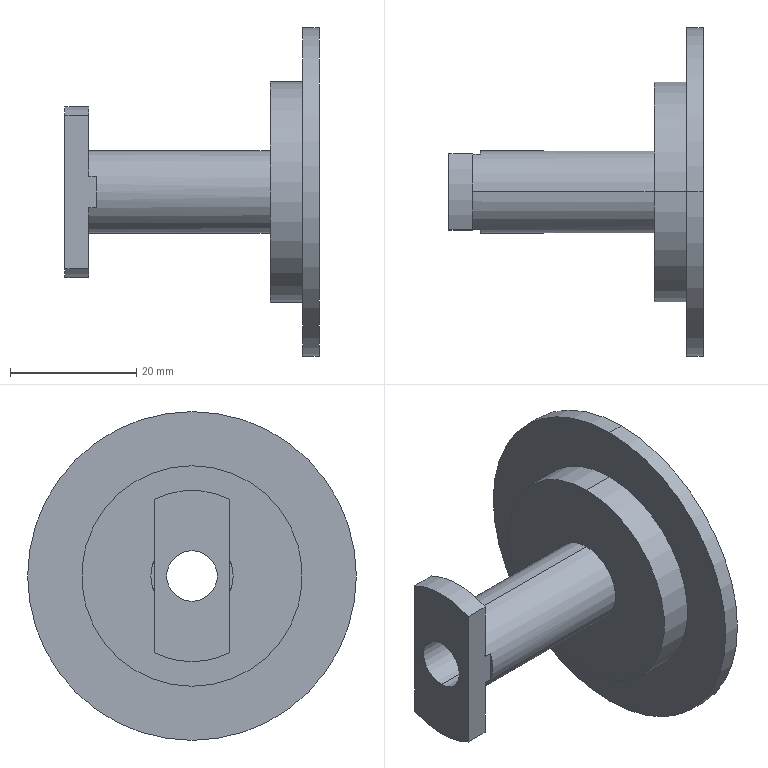Part | SolidWorks | features Cut 1, Revolution 1 | 1 solid | 24 faces | box 40.262 x 52.049 x 52.049 mm | volume 10319 mm3 | cylinder 13 | plane 11 | commonest cylinder face diameters 27.103 x3 8 x2 13.016 x2 28.307 x2 34.909 x2 52.049 x2
STEP:
#1=CARTESIAN_POINT('',(-77.,0.,14.154));
#2=VERTEX_POINT('',#1);
#3=CARTESIAN_POINT('',(-77.,0.,-14.154));
#4=VERTEX_POINT('',#3);
#5=CARTESIAN_POINT('',(-77.,0.,0.));
#6=DIRECTION('',(1.,0.,0.));
#7=DIRECTION('',(0.,0.,-1.));
#8=AXIS2_PLACEMENT_3D('',#5,#6,#7);
#9=CIRCLE('',#8,14.154);
#10=EDGE_CURVE('',#2,#4,#9,.T.);
#11=ORIENTED_EDGE('',*,*,#10,.F.);
#12=CARTESIAN_POINT('',(-71.527,0.,14.154));
#13=VERTEX_POINT('',#12);
#14=CARTESIAN_POINT('',(0.,0.,14.154));
#15=DIRECTION('',(1.,0.,0.));
#16=VECTOR('',#15,1000.);
#17=LINE('',#14,#16);
#18=EDGE_CURVE('',#2,#13,#17,.T.);
#19=ORIENTED_EDGE('',*,*,#18,.T.);
#20=CARTESIAN_POINT('',(-71.527,0.,-14.154));
#21=VERTEX_POINT('',#20);
#22=CARTESIAN_POINT('',(-71.527,0.,0.));
#23=DIRECTION('',(1.,0.,0.));
#24=DIRECTION('',(0.,0.,-1.));
#25=AXIS2_PLACEMENT_3D('',#22,#23,#24);
#26=CIRCLE('',#25,14.154);
#27=EDGE_CURVE('',#13,#21,#26,.T.);
#28=ORIENTED_EDGE('',*,*,#27,.T.);
#29=CARTESIAN_POINT('',(0.,0.,-14.154));
#30=DIRECTION('',(1.,0.,0.));
#31=VECTOR('',#30,1000.);
#32=LINE('',#29,#31);
#33=EDGE_CURVE('',#4,#21,#32,.T.);
#34=ORIENTED_EDGE('',*,*,#33,.F.);
#35=EDGE_LOOP('',(#11,#19,#28,#34));
#36=FACE_OUTER_BOUND('',#35,.T.);
#37=CARTESIAN_POINT('',(0.,0.,0.));
#38=DIRECTION('',(1.,0.,0.));
#39=DIRECTION('',(0.,0.,-1.));
#40=AXIS2_PLACEMENT_3D('',#37,#38,#39);
#41=CYLINDRICAL_SURFACE('',#40,14.154);
#42=ADVANCED_FACE('',(#36),#41,.F.);
#43=CARTESIAN_POINT('',(-111.789,0.,4.));
#44=VERTEX_POINT('',#43);
#45=CARTESIAN_POINT('',(-111.789,0.,-4.));
#46=VERTEX_POINT('',#45);
#47=CARTESIAN_POINT('',(-111.789,0.,0.));
#48=DIRECTION('',(1.,0.,0.));
#49=DIRECTION('',(0.,0.,-1.));
#50=AXIS2_PLACEMENT_3D('',#47,#48,#49);
#51=CIRCLE('',#50,4.);
#52=EDGE_CURVE('',#44,#46,#51,.T.);
#53=ORIENTED_EDGE('',*,*,#52,.F.);
#54=CARTESIAN_POINT('',(-77.,0.,4.));
#55=VERTEX_POINT('',#54);
#56=CARTESIAN_POINT('',(0.,0.,4.));
#57=DIRECTION('',(1.,0.,0.));
#58=VECTOR('',#57,1000.);
#59=LINE('',#56,#58);
#60=EDGE_CURVE('',#44,#55,#59,.T.);
#61=ORIENTED_EDGE('',*,*,#60,.T.);
#62=CARTESIAN_POINT('',(-77.,0.,-4.));
#63=VERTEX_POINT('',#62);
#64=CARTESIAN_POINT('',(-77.,0.,0.));
#65=DIRECTION('',(1.,0.,0.));
#66=DIRECTION('',(0.,0.,-1.));
#67=AXIS2_PLACEMENT_3D('',#64,#65,#66);
#68=CIRCLE('',#67,4.);
#69=EDGE_CURVE('',#55,#63,#68,.T.);
#70=ORIENTED_EDGE('',*,*,#69,.T.);
#71=CARTESIAN_POINT('',(0.,0.,-4.));
#72=DIRECTION('',(1.,0.,0.));
#73=VECTOR('',#72,1000.);
#74=LINE('',#71,#73);
#75=EDGE_CURVE('',#46,#63,#74,.T.);
#76=ORIENTED_EDGE('',*,*,#75,.F.);
#77=EDGE_LOOP('',(#53,#61,#70,#76));
#78=FACE_OUTER_BOUND('',#77,.T.);
#79=CARTESIAN_POINT('',(0.,0.,0.));
#80=DIRECTION('',(1.,0.,0.));
#81=DIRECTION('',(0.,0.,-1.));
#82=AXIS2_PLACEMENT_3D('',#79,#80,#81);
#83=CYLINDRICAL_SURFACE('',#82,4.);
#84=ADVANCED_FACE('',(#78),#83,.F.);
#85=CARTESIAN_POINT('',(-111.789,-6.,-12.151));
#86=VERTEX_POINT('',#85);
#87=CARTESIAN_POINT('',(-111.789,0.,-13.552));
#88=VERTEX_POINT('',#87);
#89=CARTESIAN_POINT('',(-111.789,0.,0.));
#90=DIRECTION('',(1.,0.,0.));
#91=DIRECTION('',(0.,0.,-1.));
#92=AXIS2_PLACEMENT_3D('',#89,#90,#91);
#93=CIRCLE('',#92,13.552);
#94=EDGE_CURVE('',#86,#88,#93,.T.);
#95=ORIENTED_EDGE('',*,*,#94,.T.);
#96=CARTESIAN_POINT('',(-108.,0.,-13.552));
#97=VERTEX_POINT('',#96);
#98=CARTESIAN_POINT('',(0.,0.,-13.552));
#99=DIRECTION('',(1.,0.,0.));
#100=VECTOR('',#99,1000.);
#101=LINE('',#98,#100);
#102=EDGE_CURVE('',#88,#97,#101,.T.);
#103=ORIENTED_EDGE('',*,*,#102,.T.);
#104=CARTESIAN_POINT('',(-108.,-6.,-12.151));
#105=VERTEX_POINT('',#104);
#106=CARTESIAN_POINT('',(-108.,0.,0.));
#107=DIRECTION('',(1.,0.,0.));
#108=DIRECTION('',(0.,0.,-1.));
#109=AXIS2_PLACEMENT_3D('',#106,#107,#108);
#110=CIRCLE('',#109,13.552);
#111=EDGE_CURVE('',#105,#97,#110,.T.);
#112=ORIENTED_EDGE('',*,*,#111,.F.);
#113=CARTESIAN_POINT('',(0.,-6.,-12.151));
#114=DIRECTION('',(1.,0.,0.));
#115=VECTOR('',#114,1000.);
#116=LINE('',#113,#115);
#117=EDGE_CURVE('',#86,#105,#116,.T.);
#118=ORIENTED_EDGE('',*,*,#117,.F.);
#119=EDGE_LOOP('',(#95,#103,#112,#118));
#120=FACE_OUTER_BOUND('',#119,.T.);
#121=CARTESIAN_POINT('',(0.,0.,0.));
#122=DIRECTION('',(1.,0.,0.));
#123=DIRECTION('',(0.,0.,-1.));
#124=AXIS2_PLACEMENT_3D('',#121,#122,#123);
#125=CYLINDRICAL_SURFACE('',#124,13.552);
#126=ADVANCED_FACE('',(#120),#125,.T.);
#127=CARTESIAN_POINT('',(-108.,6.,2.521));
#128=VERTEX_POINT('',#127);
#129=CARTESIAN_POINT('',(-108.,0.,6.508));
#130=VERTEX_POINT('',#129);
#131=CARTESIAN_POINT('',(-108.,0.,0.));
#132=DIRECTION('',(1.,0.,0.));
#133=DIRECTION('',(0.,0.,-1.));
#134=AXIS2_PLACEMENT_3D('',#131,#132,#133);
#135=CIRCLE('',#134,6.508);
#136=EDGE_CURVE('',#128,#130,#135,.T.);
#137=ORIENTED_EDGE('',*,*,#136,.T.);
#138=CARTESIAN_POINT('',(-79.307,0.,6.508));
#139=VERTEX_POINT('',#138);
#140=CARTESIAN_POINT('',(0.,0.,6.508));
#141=DIRECTION('',(1.,0.,0.));
#142=VECTOR('',#141,1000.);
#143=LINE('',#140,#142);
#144=EDGE_CURVE('',#130,#139,#143,.T.);
#145=ORIENTED_EDGE('',*,*,#144,.T.);
#146=CARTESIAN_POINT('',(-79.307,0.,-6.508));
#147=VERTEX_POINT('',#146);
#148=CARTESIAN_POINT('',(-79.307,0.,0.));
#149=DIRECTION('',(1.,0.,0.));
#150=DIRECTION('',(0.,0.,-1.));
#151=AXIS2_PLACEMENT_3D('',#148,#149,#150);
#152=CIRCLE('',#151,6.508);
#153=EDGE_CURVE('',#147,#139,#152,.T.);
#154=ORIENTED_EDGE('',*,*,#153,.F.);
#155=CARTESIAN_POINT('',(-108.,0.,-6.508));
#156=VERTEX_POINT('',#155);
#157=CARTESIAN_POINT('',(0.,0.,-6.508));
#158=DIRECTION('',(1.,0.,0.));
#159=VECTOR('',#158,1000.);
#160=LINE('',#157,#159);
#161=EDGE_CURVE('',#156,#147,#160,.T.);
#162=ORIENTED_EDGE('',*,*,#161,.F.);
#163=CARTESIAN_POINT('',(-108.,6.,-2.521));
#164=VERTEX_POINT('',#163);
#165=CARTESIAN_POINT('',(-108.,0.,0.));
#166=DIRECTION('',(1.,0.,0.));
#167=DIRECTION('',(0.,0.,-1.));
#168=AXIS2_PLACEMENT_3D('',#165,#166,#167);
#169=CIRCLE('',#168,6.508);
#170=EDGE_CURVE('',#156,#164,#169,.T.);
#171=ORIENTED_EDGE('',*,*,#170,.T.);
#172=CARTESIAN_POINT('',(-106.789,6.,-2.521));
#173=VERTEX_POINT('',#172);
#174=CARTESIAN_POINT('',(0.,6.,-2.521));
#175=DIRECTION('',(-1.,0.,0.));
#176=VECTOR('',#175,1000.);
#177=LINE('',#174,#176);
#178=EDGE_CURVE('',#173,#164,#177,.T.);
#179=ORIENTED_EDGE('',*,*,#178,.F.);
#180=CARTESIAN_POINT('',(-106.789,6.,2.521));
#181=VERTEX_POINT('',#180);
#182=CARTESIAN_POINT('',(-106.789,0.,0.));
#183=DIRECTION('',(1.,0.,0.));
#184=DIRECTION('',(0.,0.,1.));
#185=AXIS2_PLACEMENT_3D('',#182,#183,#184);
#186=CIRCLE('',#185,6.508);
#187=EDGE_CURVE('',#173,#181,#186,.T.);
#188=ORIENTED_EDGE('',*,*,#187,.T.);
#189=CARTESIAN_POINT('',(0.,6.,2.521));
#190=DIRECTION('',(1.,0.,0.));
#191=VECTOR('',#190,1000.);
#192=LINE('',#189,#191);
#193=EDGE_CURVE('',#128,#181,#192,.T.);
#194=ORIENTED_EDGE('',*,*,#193,.F.);
#195=EDGE_LOOP('',(#137,#145,#154,#162,#171,#179,#188,#194));
#196=FACE_OUTER_BOUND('',#195,.T.);
#197=CARTESIAN_POINT('',(0.,0.,0.));
#198=DIRECTION('',(1.,0.,0.));
#199=DIRECTION('',(0.,0.,-1.));
#200=AXIS2_PLACEMENT_3D('',#197,#198,#199);
#201=CYLINDRICAL_SURFACE('',#200,6.508);
#202=ADVANCED_FACE('',(#196),#201,.T.);
#203=CARTESIAN_POINT('',(-79.307,0.,-17.455));
#204=VERTEX_POINT('',#203);
#205=CARTESIAN_POINT('',(-79.307,0.,17.455));
#206=VERTEX_POINT('',#205);
#207=CARTESIAN_POINT('',(-79.307,0.,0.));
#208=DIRECTION('',(1.,0.,0.));
#209=DIRECTION('',(0.,0.,-1.));
#210=AXIS2_PLACEMENT_3D('',#207,#208,#209);
#211=CIRCLE('',#210,17.455);
#212=EDGE_CURVE('',#204,#206,#211,.T.);
#213=ORIENTED_EDGE('',*,*,#212,.T.);
#214=CARTESIAN_POINT('',(-74.143,0.,17.455));
#215=VERTEX_POINT('',#214);
#216=CARTESIAN_POINT('',(0.,0.,17.455));
#217=DIRECTION('',(1.,0.,0.));
#218=VECTOR('',#217,1000.);
#219=LINE('',#216,#218);
#220=EDGE_CURVE('',#206,#215,#219,.T.);
#221=ORIENTED_EDGE('',*,*,#220,.T.);
#222=CARTESIAN_POINT('',(-74.143,0.,-17.455));
#223=VERTEX_POINT('',#222);
#224=CARTESIAN_POINT('',(-74.143,0.,0.));
#225=DIRECTION('',(1.,0.,0.));
#226=DIRECTION('',(0.,0.,-1.));
#227=AXIS2_PLACEMENT_3D('',#224,#225,#226);
#228=CIRCLE('',#227,17.455);
#229=EDGE_CURVE('',#223,#215,#228,.T.);
#230=ORIENTED_EDGE('',*,*,#229,.F.);
#231=CARTESIAN_POINT('',(0.,0.,-17.455));
#232=DIRECTION('',(1.,0.,0.));
#233=VECTOR('',#232,1000.);
#234=LINE('',#231,#233);
#235=EDGE_CURVE('',#204,#223,#234,.T.);
#236=ORIENTED_EDGE('',*,*,#235,.F.);
#237=EDGE_LOOP('',(#213,#221,#230,#236));
#238=FACE_OUTER_BOUND('',#237,.T.);
#239=CARTESIAN_POINT('',(0.,0.,0.));
#240=DIRECTION('',(1.,0.,0.));
#241=DIRECTION('',(0.,0.,-1.));
#242=AXIS2_PLACEMENT_3D('',#239,#240,#241);
#243=CYLINDRICAL_SURFACE('',#242,17.455);
#244=ADVANCED_FACE('',(#238),#243,.T.);
#245=CARTESIAN_POINT('',(-74.143,0.,-26.024));
#246=VERTEX_POINT('',#245);
#247=CARTESIAN_POINT('',(-74.143,0.,26.024));
#248=VERTEX_POINT('',#247);
#249=CARTESIAN_POINT('',(-74.143,0.,0.));
#250=DIRECTION('',(1.,0.,0.));
#251=DIRECTION('',(0.,0.,-1.));
#252=AXIS2_PLACEMENT_3D('',#249,#250,#251);
#253=CIRCLE('',#252,26.024);
#254=EDGE_CURVE('',#246,#248,#253,.T.);
#255=ORIENTED_EDGE('',*,*,#254,.T.);
#256=CARTESIAN_POINT('',(-71.527,0.,26.024));
#257=VERTEX_POINT('',#256);
#258=CARTESIAN_POINT('',(0.,0.,26.024));
#259=DIRECTION('',(1.,0.,0.));
#260=VECTOR('',#259,1000.);
#261=LINE('',#258,#260);
#262=EDGE_CURVE('',#248,#257,#261,.T.);
#263=ORIENTED_EDGE('',*,*,#262,.T.);
#264=CARTESIAN_POINT('',(-71.527,0.,-26.024));
#265=VERTEX_POINT('',#264);
#266=CARTESIAN_POINT('',(-71.527,0.,0.));
#267=DIRECTION('',(1.,0.,0.));
#268=DIRECTION('',(0.,0.,-1.));
#269=AXIS2_PLACEMENT_3D('',#266,#267,#268);
#270=CIRCLE('',#269,26.024);
#271=EDGE_CURVE('',#265,#257,#270,.T.);
#272=ORIENTED_EDGE('',*,*,#271,.F.);
#273=CARTESIAN_POINT('',(0.,0.,-26.024));
#274=DIRECTION('',(1.,0.,0.));
#275=VECTOR('',#274,1000.);
#276=LINE('',#273,#275);
#277=EDGE_CURVE('',#246,#265,#276,.T.);
#278=ORIENTED_EDGE('',*,*,#277,.F.);
#279=EDGE_LOOP('',(#255,#263,#272,#278));
#280=FACE_OUTER_BOUND('',#279,.T.);
#281=CARTESIAN_POINT('',(0.,0.,0.));
#282=DIRECTION('',(1.,0.,0.));
#283=DIRECTION('',(0.,0.,-1.));
#284=AXIS2_PLACEMENT_3D('',#281,#282,#283);
#285=CYLINDRICAL_SURFACE('',#284,26.024);
#286=ADVANCED_FACE('',(#280),#285,.T.);
#287=CARTESIAN_POINT('',(-108.,-6.,-2.521));
#288=VERTEX_POINT('',#287);
#289=CARTESIAN_POINT('',(-108.,-6.,0.));
#290=DIRECTION('',(0.,0.,1.));
#291=VECTOR('',#290,1000.);
#292=LINE('',#289,#291);
#293=EDGE_CURVE('',#105,#288,#292,.T.);
#294=ORIENTED_EDGE('',*,*,#293,.F.);
#295=ORIENTED_EDGE('',*,*,#111,.T.);
#296=CARTESIAN_POINT('',(-108.,6.,-12.151));
#297=VERTEX_POINT('',#296);
#298=CARTESIAN_POINT('',(-108.,0.,0.));
#299=DIRECTION('',(1.,0.,0.));
#300=DIRECTION('',(0.,0.,-1.));
#301=AXIS2_PLACEMENT_3D('',#298,#299,#300);
#302=CIRCLE('',#301,13.552);
#303=EDGE_CURVE('',#97,#297,#302,.T.);
#304=ORIENTED_EDGE('',*,*,#303,.T.);
#305=CARTESIAN_POINT('',(-108.,6.,0.));
#306=DIRECTION('',(0.,0.,-1.));
#307=VECTOR('',#306,1000.);
#308=LINE('',#305,#307);
#309=EDGE_CURVE('',#164,#297,#308,.T.);
#310=ORIENTED_EDGE('',*,*,#309,.F.);
#311=ORIENTED_EDGE('',*,*,#170,.F.);
#312=CARTESIAN_POINT('',(-108.,0.,0.));
#313=DIRECTION('',(1.,0.,0.));
#314=DIRECTION('',(0.,0.,-1.));
#315=AXIS2_PLACEMENT_3D('',#312,#313,#314);
#316=CIRCLE('',#315,6.508);
#317=EDGE_CURVE('',#288,#156,#316,.T.);
#318=ORIENTED_EDGE('',*,*,#317,.F.);
#319=EDGE_LOOP('',(#294,#295,#304,#310,#311,#318));
#320=FACE_OUTER_BOUND('',#319,.T.);
#321=CARTESIAN_POINT('',(-108.,6.508,0.));
#322=DIRECTION('',(1.,0.,0.));
#323=DIRECTION('',(0.,0.,-1.));
#324=AXIS2_PLACEMENT_3D('',#321,#322,#323);
#325=PLANE('',#324);
#326=ADVANCED_FACE('',(#320),#325,.T.);
#327=CARTESIAN_POINT('',(-108.,-6.,12.151));
#328=VERTEX_POINT('',#327);
#329=CARTESIAN_POINT('',(-111.789,-6.,12.151));
#330=VERTEX_POINT('',#329);
#331=CARTESIAN_POINT('',(0.,-6.,12.151));
#332=DIRECTION('',(-1.,0.,0.));
#333=VECTOR('',#332,1000.);
#334=LINE('',#331,#333);
#335=EDGE_CURVE('',#328,#330,#334,.T.);
#336=ORIENTED_EDGE('',*,*,#335,.F.);
#337=CARTESIAN_POINT('',(-108.,6.,12.151));
#338=VERTEX_POINT('',#337);
#339=CARTESIAN_POINT('',(-108.,0.,0.));
#340=DIRECTION('',(1.,0.,0.));
#341=DIRECTION('',(0.,0.,-1.));
#342=AXIS2_PLACEMENT_3D('',#339,#340,#341);
#343=CIRCLE('',#342,13.552);
#344=EDGE_CURVE('',#338,#328,#343,.T.);
#345=ORIENTED_EDGE('',*,*,#344,.F.);
#346=CARTESIAN_POINT('',(-111.789,6.,12.151));
#347=VERTEX_POINT('',#346);
#348=CARTESIAN_POINT('',(0.,6.,12.151));
#349=DIRECTION('',(1.,0.,0.));
#350=VECTOR('',#349,1000.);
#351=LINE('',#348,#350);
#352=EDGE_CURVE('',#347,#338,#351,.T.);
#353=ORIENTED_EDGE('',*,*,#352,.F.);
#354=CARTESIAN_POINT('',(-111.789,0.,0.));
#355=DIRECTION('',(1.,0.,0.));
#356=DIRECTION('',(0.,0.,-1.));
#357=AXIS2_PLACEMENT_3D('',#354,#355,#356);
#358=CIRCLE('',#357,13.552);
#359=EDGE_CURVE('',#347,#330,#358,.T.);
#360=ORIENTED_EDGE('',*,*,#359,.T.);
#361=EDGE_LOOP('',(#336,#345,#353,#360));
#362=FACE_OUTER_BOUND('',#361,.T.);
#363=CARTESIAN_POINT('',(0.,0.,0.));
#364=DIRECTION('',(1.,0.,0.));
#365=DIRECTION('',(0.,0.,-1.));
#366=AXIS2_PLACEMENT_3D('',#363,#364,#365);
#367=CYLINDRICAL_SURFACE('',#366,13.552);
#368=ADVANCED_FACE('',(#362),#367,.T.);
#369=ORIENTED_EDGE('',*,*,#262,.F.);
#370=CARTESIAN_POINT('',(-74.143,0.,0.));
#371=DIRECTION('',(1.,0.,0.));
#372=DIRECTION('',(0.,0.,-1.));
#373=AXIS2_PLACEMENT_3D('',#370,#371,#372);
#374=CIRCLE('',#373,26.024);
#375=EDGE_CURVE('',#248,#246,#374,.T.);
#376=ORIENTED_EDGE('',*,*,#375,.T.);
#377=ORIENTED_EDGE('',*,*,#277,.T.);
#378=CARTESIAN_POINT('',(-71.527,0.,0.));
#379=DIRECTION('',(1.,0.,0.));
#380=DIRECTION('',(0.,0.,-1.));
#381=AXIS2_PLACEMENT_3D('',#378,#379,#380);
#382=CIRCLE('',#381,26.024);
#383=EDGE_CURVE('',#257,#265,#382,.T.);
#384=ORIENTED_EDGE('',*,*,#383,.F.);
#385=EDGE_LOOP('',(#369,#376,#377,#384));
#386=FACE_OUTER_BOUND('',#385,.T.);
#387=CARTESIAN_POINT('',(0.,0.,0.));
#388=DIRECTION('',(1.,0.,0.));
#389=DIRECTION('',(0.,0.,-1.));
#390=AXIS2_PLACEMENT_3D('',#387,#388,#389);
#391=CYLINDRICAL_SURFACE('',#390,26.024);
#392=ADVANCED_FACE('',(#386),#391,.T.);
#393=ORIENTED_EDGE('',*,*,#229,.T.);
#394=CARTESIAN_POINT('',(-74.143,0.,0.));
#395=DIRECTION('',(1.,0.,0.));
#396=DIRECTION('',(0.,0.,-1.));
#397=AXIS2_PLACEMENT_3D('',#394,#395,#396);
#398=CIRCLE('',#397,17.455);
#399=EDGE_CURVE('',#215,#223,#398,.T.);
#400=ORIENTED_EDGE('',*,*,#399,.T.);
#401=EDGE_LOOP('',(#393,#400));
#402=FACE_BOUND('',#401,.T.);
#403=ORIENTED_EDGE('',*,*,#254,.F.);
#404=ORIENTED_EDGE('',*,*,#375,.F.);
#405=EDGE_LOOP('',(#403,#404));
#406=FACE_OUTER_BOUND('',#405,.T.);
#407=CARTESIAN_POINT('',(-74.143,26.024,0.));
#408=DIRECTION('',(-1.,0.,0.));
#409=DIRECTION('',(0.,0.,1.));
#410=AXIS2_PLACEMENT_3D('',#407,#408,#409);
#411=PLANE('',#410);
#412=ADVANCED_FACE('',(#402,#406),#411,.T.);
#413=ORIENTED_EDGE('',*,*,#220,.F.);
#414=CARTESIAN_POINT('',(-79.307,0.,0.));
#415=DIRECTION('',(1.,0.,0.));
#416=DIRECTION('',(0.,0.,-1.));
#417=AXIS2_PLACEMENT_3D('',#414,#415,#416);
#418=CIRCLE('',#417,17.455);
#419=EDGE_CURVE('',#206,#204,#418,.T.);
#420=ORIENTED_EDGE('',*,*,#419,.T.);
#421=ORIENTED_EDGE('',*,*,#235,.T.);
#422=ORIENTED_EDGE('',*,*,#399,.F.);
#423=EDGE_LOOP('',(#413,#420,#421,#422));
#424=FACE_OUTER_BOUND('',#423,.T.);
#425=CARTESIAN_POINT('',(0.,0.,0.));
#426=DIRECTION('',(1.,0.,0.));
#427=DIRECTION('',(0.,0.,-1.));
#428=AXIS2_PLACEMENT_3D('',#425,#426,#427);
#429=CYLINDRICAL_SURFACE('',#428,17.455);
#430=ADVANCED_FACE('',(#424),#429,.T.);
#431=ORIENTED_EDGE('',*,*,#153,.T.);
#432=CARTESIAN_POINT('',(-79.307,0.,0.));
#433=DIRECTION('',(1.,0.,0.));
#434=DIRECTION('',(0.,0.,-1.));
#435=AXIS2_PLACEMENT_3D('',#432,#433,#434);
#436=CIRCLE('',#435,6.508);
#437=EDGE_CURVE('',#139,#147,#436,.T.);
#438=ORIENTED_EDGE('',*,*,#437,.T.);
#439=EDGE_LOOP('',(#431,#438));
#440=FACE_BOUND('',#439,.T.);
#441=ORIENTED_EDGE('',*,*,#212,.F.);
#442=ORIENTED_EDGE('',*,*,#419,.F.);
#443=EDGE_LOOP('',(#441,#442));
#444=FACE_OUTER_BOUND('',#443,.T.);
#445=CARTESIAN_POINT('',(-79.307,17.455,0.));
#446=DIRECTION('',(-1.,0.,0.));
#447=DIRECTION('',(0.,0.,1.));
#448=AXIS2_PLACEMENT_3D('',#445,#446,#447);
#449=PLANE('',#448);
#450=ADVANCED_FACE('',(#440,#444),#449,.T.);
#451=ORIENTED_EDGE('',*,*,#144,.F.);
#452=CARTESIAN_POINT('',(-108.,-6.,2.521));
#453=VERTEX_POINT('',#452);
#454=CARTESIAN_POINT('',(-108.,0.,0.));
#455=DIRECTION('',(1.,0.,0.));
#456=DIRECTION('',(0.,0.,-1.));
#457=AXIS2_PLACEMENT_3D('',#454,#455,#456);
#458=CIRCLE('',#457,6.508);
#459=EDGE_CURVE('',#130,#453,#458,.T.);
#460=ORIENTED_EDGE('',*,*,#459,.T.);
#461=CARTESIAN_POINT('',(-106.789,-6.,2.521));
#462=VERTEX_POINT('',#461);
#463=CARTESIAN_POINT('',(0.,-6.,2.521));
#464=DIRECTION('',(-1.,0.,0.));
#465=VECTOR('',#464,1000.);
#466=LINE('',#463,#465);
#467=EDGE_CURVE('',#462,#453,#466,.T.);
#468=ORIENTED_EDGE('',*,*,#467,.F.);
#469=CARTESIAN_POINT('',(-106.789,-6.,-2.521));
#470=VERTEX_POINT('',#469);
#471=CARTESIAN_POINT('',(-106.789,0.,0.));
#472=DIRECTION('',(-1.,0.,0.));
#473=DIRECTION('',(0.,0.,-1.));
#474=AXIS2_PLACEMENT_3D('',#471,#472,#473);
#475=CIRCLE('',#474,6.508);
#476=EDGE_CURVE('',#470,#462,#475,.T.);
#477=ORIENTED_EDGE('',*,*,#476,.F.);
#478=CARTESIAN_POINT('',(0.,-6.,-2.521));
#479=DIRECTION('',(1.,0.,0.));
#480=VECTOR('',#479,1000.);
#481=LINE('',#478,#480);
#482=EDGE_CURVE('',#288,#470,#481,.T.);
#483=ORIENTED_EDGE('',*,*,#482,.F.);
#484=ORIENTED_EDGE('',*,*,#317,.T.);
#485=ORIENTED_EDGE('',*,*,#161,.T.);
#486=ORIENTED_EDGE('',*,*,#437,.F.);
#487=EDGE_LOOP('',(#451,#460,#468,#477,#483,#484,#485,#486));
#488=FACE_OUTER_BOUND('',#487,.T.);
#489=CARTESIAN_POINT('',(0.,0.,0.));
#490=DIRECTION('',(1.,0.,0.));
#491=DIRECTION('',(0.,0.,-1.));
#492=AXIS2_PLACEMENT_3D('',#489,#490,#491);
#493=CYLINDRICAL_SURFACE('',#492,6.508);
#494=ADVANCED_FACE('',(#488),#493,.T.);
#495=CARTESIAN_POINT('',(-108.,-6.,0.));
#496=DIRECTION('',(0.,0.,1.));
#497=VECTOR('',#496,1000.);
#498=LINE('',#495,#497);
#499=EDGE_CURVE('',#453,#328,#498,.T.);
#500=ORIENTED_EDGE('',*,*,#499,.F.);
#501=ORIENTED_EDGE('',*,*,#459,.F.);
#502=ORIENTED_EDGE('',*,*,#136,.F.);
#503=CARTESIAN_POINT('',(-108.,6.,0.));
#504=DIRECTION('',(0.,0.,-1.));
#505=VECTOR('',#504,1000.);
#506=LINE('',#503,#505);
#507=EDGE_CURVE('',#338,#128,#506,.T.);
#508=ORIENTED_EDGE('',*,*,#507,.F.);
#509=ORIENTED_EDGE('',*,*,#344,.T.);
#510=EDGE_LOOP('',(#500,#501,#502,#508,#509));
#511=FACE_OUTER_BOUND('',#510,.T.);
#512=CARTESIAN_POINT('',(-108.,6.508,0.));
#513=DIRECTION('',(1.,0.,0.));
#514=DIRECTION('',(0.,0.,-1.));
#515=AXIS2_PLACEMENT_3D('',#512,#513,#514);
#516=PLANE('',#515);
#517=ADVANCED_FACE('',(#511),#516,.T.);
#518=ORIENTED_EDGE('',*,*,#102,.F.);
#519=CARTESIAN_POINT('',(-111.789,6.,-12.151));
#520=VERTEX_POINT('',#519);
#521=CARTESIAN_POINT('',(-111.789,0.,0.));
#522=DIRECTION('',(1.,0.,0.));
#523=DIRECTION('',(0.,0.,-1.));
#524=AXIS2_PLACEMENT_3D('',#521,#522,#523);
#525=CIRCLE('',#524,13.552);
#526=EDGE_CURVE('',#88,#520,#525,.T.);
#527=ORIENTED_EDGE('',*,*,#526,.T.);
#528=CARTESIAN_POINT('',(0.,6.,-12.151));
#529=DIRECTION('',(-1.,0.,0.));
#530=VECTOR('',#529,1000.);
#531=LINE('',#528,#530);
#532=EDGE_CURVE('',#297,#520,#531,.T.);
#533=ORIENTED_EDGE('',*,*,#532,.F.);
#534=ORIENTED_EDGE('',*,*,#303,.F.);
#535=EDGE_LOOP('',(#518,#527,#533,#534));
#536=FACE_OUTER_BOUND('',#535,.T.);
#537=CARTESIAN_POINT('',(0.,0.,0.));
#538=DIRECTION('',(1.,0.,0.));
#539=DIRECTION('',(0.,0.,-1.));
#540=AXIS2_PLACEMENT_3D('',#537,#538,#539);
#541=CYLINDRICAL_SURFACE('',#540,13.552);
#542=ADVANCED_FACE('',(#536),#541,.T.);
#543=CARTESIAN_POINT('',(-111.789,-6.,0.));
#544=DIRECTION('',(0.,0.,-1.));
#545=VECTOR('',#544,1000.);
#546=LINE('',#543,#545);
#547=EDGE_CURVE('',#330,#86,#546,.T.);
#548=ORIENTED_EDGE('',*,*,#547,.F.);
#549=ORIENTED_EDGE('',*,*,#359,.F.);
#550=CARTESIAN_POINT('',(-111.789,6.,0.));
#551=DIRECTION('',(0.,0.,1.));
#552=VECTOR('',#551,1000.);
#553=LINE('',#550,#552);
#554=EDGE_CURVE('',#520,#347,#553,.T.);
#555=ORIENTED_EDGE('',*,*,#554,.F.);
#556=ORIENTED_EDGE('',*,*,#526,.F.);
#557=ORIENTED_EDGE('',*,*,#94,.F.);
#558=EDGE_LOOP('',(#548,#549,#555,#556,#557));
#559=FACE_OUTER_BOUND('',#558,.T.);
#560=CARTESIAN_POINT('',(-111.789,0.,0.));
#561=DIRECTION('',(1.,0.,0.));
#562=DIRECTION('',(0.,0.,-1.));
#563=AXIS2_PLACEMENT_3D('',#560,#561,#562);
#564=CIRCLE('',#563,4.);
#565=EDGE_CURVE('',#46,#44,#564,.T.);
#566=ORIENTED_EDGE('',*,*,#565,.T.);
#567=ORIENTED_EDGE('',*,*,#52,.T.);
#568=EDGE_LOOP('',(#566,#567));
#569=FACE_BOUND('',#568,.T.);
#570=CARTESIAN_POINT('',(-111.789,13.552,0.));
#571=DIRECTION('',(-1.,0.,0.));
#572=DIRECTION('',(0.,0.,1.));
#573=AXIS2_PLACEMENT_3D('',#570,#571,#572);
#574=PLANE('',#573);
#575=ADVANCED_FACE('',(#559,#569),#574,.T.);
#576=ORIENTED_EDGE('',*,*,#60,.F.);
#577=ORIENTED_EDGE('',*,*,#565,.F.);
#578=ORIENTED_EDGE('',*,*,#75,.T.);
#579=CARTESIAN_POINT('',(-77.,0.,0.));
#580=DIRECTION('',(1.,0.,0.));
#581=DIRECTION('',(0.,0.,-1.));
#582=AXIS2_PLACEMENT_3D('',#579,#580,#581);
#583=CIRCLE('',#582,4.);
#584=EDGE_CURVE('',#63,#55,#583,.T.);
#585=ORIENTED_EDGE('',*,*,#584,.T.);
#586=EDGE_LOOP('',(#576,#577,#578,#585));
#587=FACE_OUTER_BOUND('',#586,.T.);
#588=CARTESIAN_POINT('',(0.,0.,0.));
#589=DIRECTION('',(1.,0.,0.));
#590=DIRECTION('',(0.,0.,-1.));
#591=AXIS2_PLACEMENT_3D('',#588,#589,#590);
#592=CYLINDRICAL_SURFACE('',#591,4.);
#593=ADVANCED_FACE('',(#587),#592,.F.);
#594=CARTESIAN_POINT('',(-77.,0.,0.));
#595=DIRECTION('',(1.,0.,0.));
#596=DIRECTION('',(0.,0.,-1.));
#597=AXIS2_PLACEMENT_3D('',#594,#595,#596);
#598=CIRCLE('',#597,14.154);
#599=EDGE_CURVE('',#4,#2,#598,.T.);
#600=ORIENTED_EDGE('',*,*,#599,.T.);
#601=ORIENTED_EDGE('',*,*,#10,.T.);
#602=EDGE_LOOP('',(#600,#601));
#603=FACE_OUTER_BOUND('',#602,.T.);
#604=ORIENTED_EDGE('',*,*,#584,.F.);
#605=ORIENTED_EDGE('',*,*,#69,.F.);
#606=EDGE_LOOP('',(#604,#605));
#607=FACE_BOUND('',#606,.T.);
#608=CARTESIAN_POINT('',(-77.,4.,0.));
#609=DIRECTION('',(1.,0.,0.));
#610=DIRECTION('',(0.,0.,-1.));
#611=AXIS2_PLACEMENT_3D('',#608,#609,#610);
#612=PLANE('',#611);
#613=ADVANCED_FACE('',(#603,#607),#612,.T.);
#614=ORIENTED_EDGE('',*,*,#18,.F.);
#615=ORIENTED_EDGE('',*,*,#599,.F.);
#616=ORIENTED_EDGE('',*,*,#33,.T.);
#617=CARTESIAN_POINT('',(-71.527,0.,0.));
#618=DIRECTION('',(1.,0.,0.));
#619=DIRECTION('',(0.,0.,-1.));
#620=AXIS2_PLACEMENT_3D('',#617,#618,#619);
#621=CIRCLE('',#620,14.154);
#622=EDGE_CURVE('',#21,#13,#621,.T.);
#623=ORIENTED_EDGE('',*,*,#622,.T.);
#624=EDGE_LOOP('',(#614,#615,#616,#623));
#625=FACE_OUTER_BOUND('',#624,.T.);
#626=CARTESIAN_POINT('',(0.,0.,0.));
#627=DIRECTION('',(1.,0.,0.));
#628=DIRECTION('',(0.,0.,-1.));
#629=AXIS2_PLACEMENT_3D('',#626,#627,#628);
#630=CYLINDRICAL_SURFACE('',#629,14.154);
#631=ADVANCED_FACE('',(#625),#630,.F.);
#632=ORIENTED_EDGE('',*,*,#271,.T.);
#633=ORIENTED_EDGE('',*,*,#383,.T.);
#634=EDGE_LOOP('',(#632,#633));
#635=FACE_OUTER_BOUND('',#634,.T.);
#636=ORIENTED_EDGE('',*,*,#622,.F.);
#637=ORIENTED_EDGE('',*,*,#27,.F.);
#638=EDGE_LOOP('',(#636,#637));
#639=FACE_BOUND('',#638,.T.);
#640=CARTESIAN_POINT('',(-71.527,14.154,0.));
#641=DIRECTION('',(1.,0.,0.));
#642=DIRECTION('',(0.,0.,-1.));
#643=AXIS2_PLACEMENT_3D('',#640,#641,#642);
#644=PLANE('',#643);
#645=ADVANCED_FACE('',(#635,#639),#644,.T.);
#646=ORIENTED_EDGE('',*,*,#178,.T.);
#647=ORIENTED_EDGE('',*,*,#309,.T.);
#648=ORIENTED_EDGE('',*,*,#532,.T.);
#649=ORIENTED_EDGE('',*,*,#554,.T.);
#650=ORIENTED_EDGE('',*,*,#352,.T.);
#651=ORIENTED_EDGE('',*,*,#507,.T.);
#652=ORIENTED_EDGE('',*,*,#193,.T.);
#653=CARTESIAN_POINT('',(-106.789,6.,-44.604));
#654=DIRECTION('',(0.,0.,1.));
#655=VECTOR('',#654,1000.);
#656=LINE('',#653,#655);
#657=EDGE_CURVE('',#173,#181,#656,.T.);
#658=ORIENTED_EDGE('',*,*,#657,.F.);
#659=EDGE_LOOP('',(#646,#647,#648,#649,#650,#651,#652,#658));
#660=FACE_OUTER_BOUND('',#659,.T.);
#661=CARTESIAN_POINT('',(-106.789,6.,-44.604));
#662=DIRECTION('',(0.,-1.,0.));
#663=DIRECTION('',(0.,0.,-1.));
#664=AXIS2_PLACEMENT_3D('',#661,#662,#663);
#665=PLANE('',#664);
#666=ADVANCED_FACE('',(#660),#665,.F.);
#667=ORIENTED_EDGE('',*,*,#657,.T.);
#668=ORIENTED_EDGE('',*,*,#187,.F.);
#669=EDGE_LOOP('',(#667,#668));
#670=FACE_OUTER_BOUND('',#669,.T.);
#671=CARTESIAN_POINT('',(-106.789,0.,0.));
#672=DIRECTION('',(-1.,0.,0.));
#673=DIRECTION('',(0.,0.,1.));
#674=AXIS2_PLACEMENT_3D('',#671,#672,#673);
#675=PLANE('',#674);
#676=ADVANCED_FACE('',(#670),#675,.T.);
#677=ORIENTED_EDGE('',*,*,#467,.T.);
#678=ORIENTED_EDGE('',*,*,#499,.T.);
#679=ORIENTED_EDGE('',*,*,#335,.T.);
#680=ORIENTED_EDGE('',*,*,#547,.T.);
#681=ORIENTED_EDGE('',*,*,#117,.T.);
#682=ORIENTED_EDGE('',*,*,#293,.T.);
#683=ORIENTED_EDGE('',*,*,#482,.T.);
#684=CARTESIAN_POINT('',(-106.789,-6.,79.996));
#685=DIRECTION('',(0.,0.,-1.));
#686=VECTOR('',#685,1000.);
#687=LINE('',#684,#686);
#688=EDGE_CURVE('',#462,#470,#687,.T.);
#689=ORIENTED_EDGE('',*,*,#688,.F.);
#690=EDGE_LOOP('',(#677,#678,#679,#680,#681,#682,#683,#689));
#691=FACE_OUTER_BOUND('',#690,.T.);
#692=CARTESIAN_POINT('',(-106.789,-6.,79.996));
#693=DIRECTION('',(0.,1.,0.));
#694=DIRECTION('',(0.,0.,1.));
#695=AXIS2_PLACEMENT_3D('',#692,#693,#694);
#696=PLANE('',#695);
#697=ADVANCED_FACE('',(#691),#696,.F.);
#698=ORIENTED_EDGE('',*,*,#476,.T.);
#699=ORIENTED_EDGE('',*,*,#688,.T.);
#700=EDGE_LOOP('',(#698,#699));
#701=FACE_OUTER_BOUND('',#700,.T.);
#702=CARTESIAN_POINT('',(-106.789,0.,0.));
#703=DIRECTION('',(1.,0.,0.));
#704=DIRECTION('',(0.,0.,-1.));
#705=AXIS2_PLACEMENT_3D('',#702,#703,#704);
#706=PLANE('',#705);
#707=ADVANCED_FACE('',(#701),#706,.F.);
#708=CLOSED_SHELL('',(#42,#84,#126,#202,#244,#286,#326,#368,#392,#412,#430,#450,#494,#517,#542,#575,#593,#613,#631,#645,#666,#676,#697,#707));
#709=MANIFOLD_SOLID_BREP('',#708);
#710=CARTESIAN_POINT('',(0.,0.,0.));
#711=DIRECTION('',(0.,0.,1.));
#712=DIRECTION('',(1.,0.,0.));
#713=AXIS2_PLACEMENT_3D('',#710,#711,#712);
#714=(LENGTH_UNIT()NAMED_UNIT(*)SI_UNIT(.MILLI.,.METRE.));
#715=UNCERTAINTY_MEASURE_WITH_UNIT(LENGTH_MEASURE(0.00001),#714,'','');
#716=(NAMED_UNIT(*)PLANE_ANGLE_UNIT()SI_UNIT($,.RADIAN.));
#717=(NAMED_UNIT(*)SI_UNIT($,.STERADIAN.)SOLID_ANGLE_UNIT());
#718=(GEOMETRIC_REPRESENTATION_CONTEXT(3)GLOBAL_UNCERTAINTY_ASSIGNED_CONTEXT((#715))GLOBAL_UNIT_ASSIGNED_CONTEXT((#714,#716,#717))REPRESENTATION_CONTEXT('',''));
#719=ADVANCED_BREP_SHAPE_REPRESENTATION('',(#709,#713),#718);